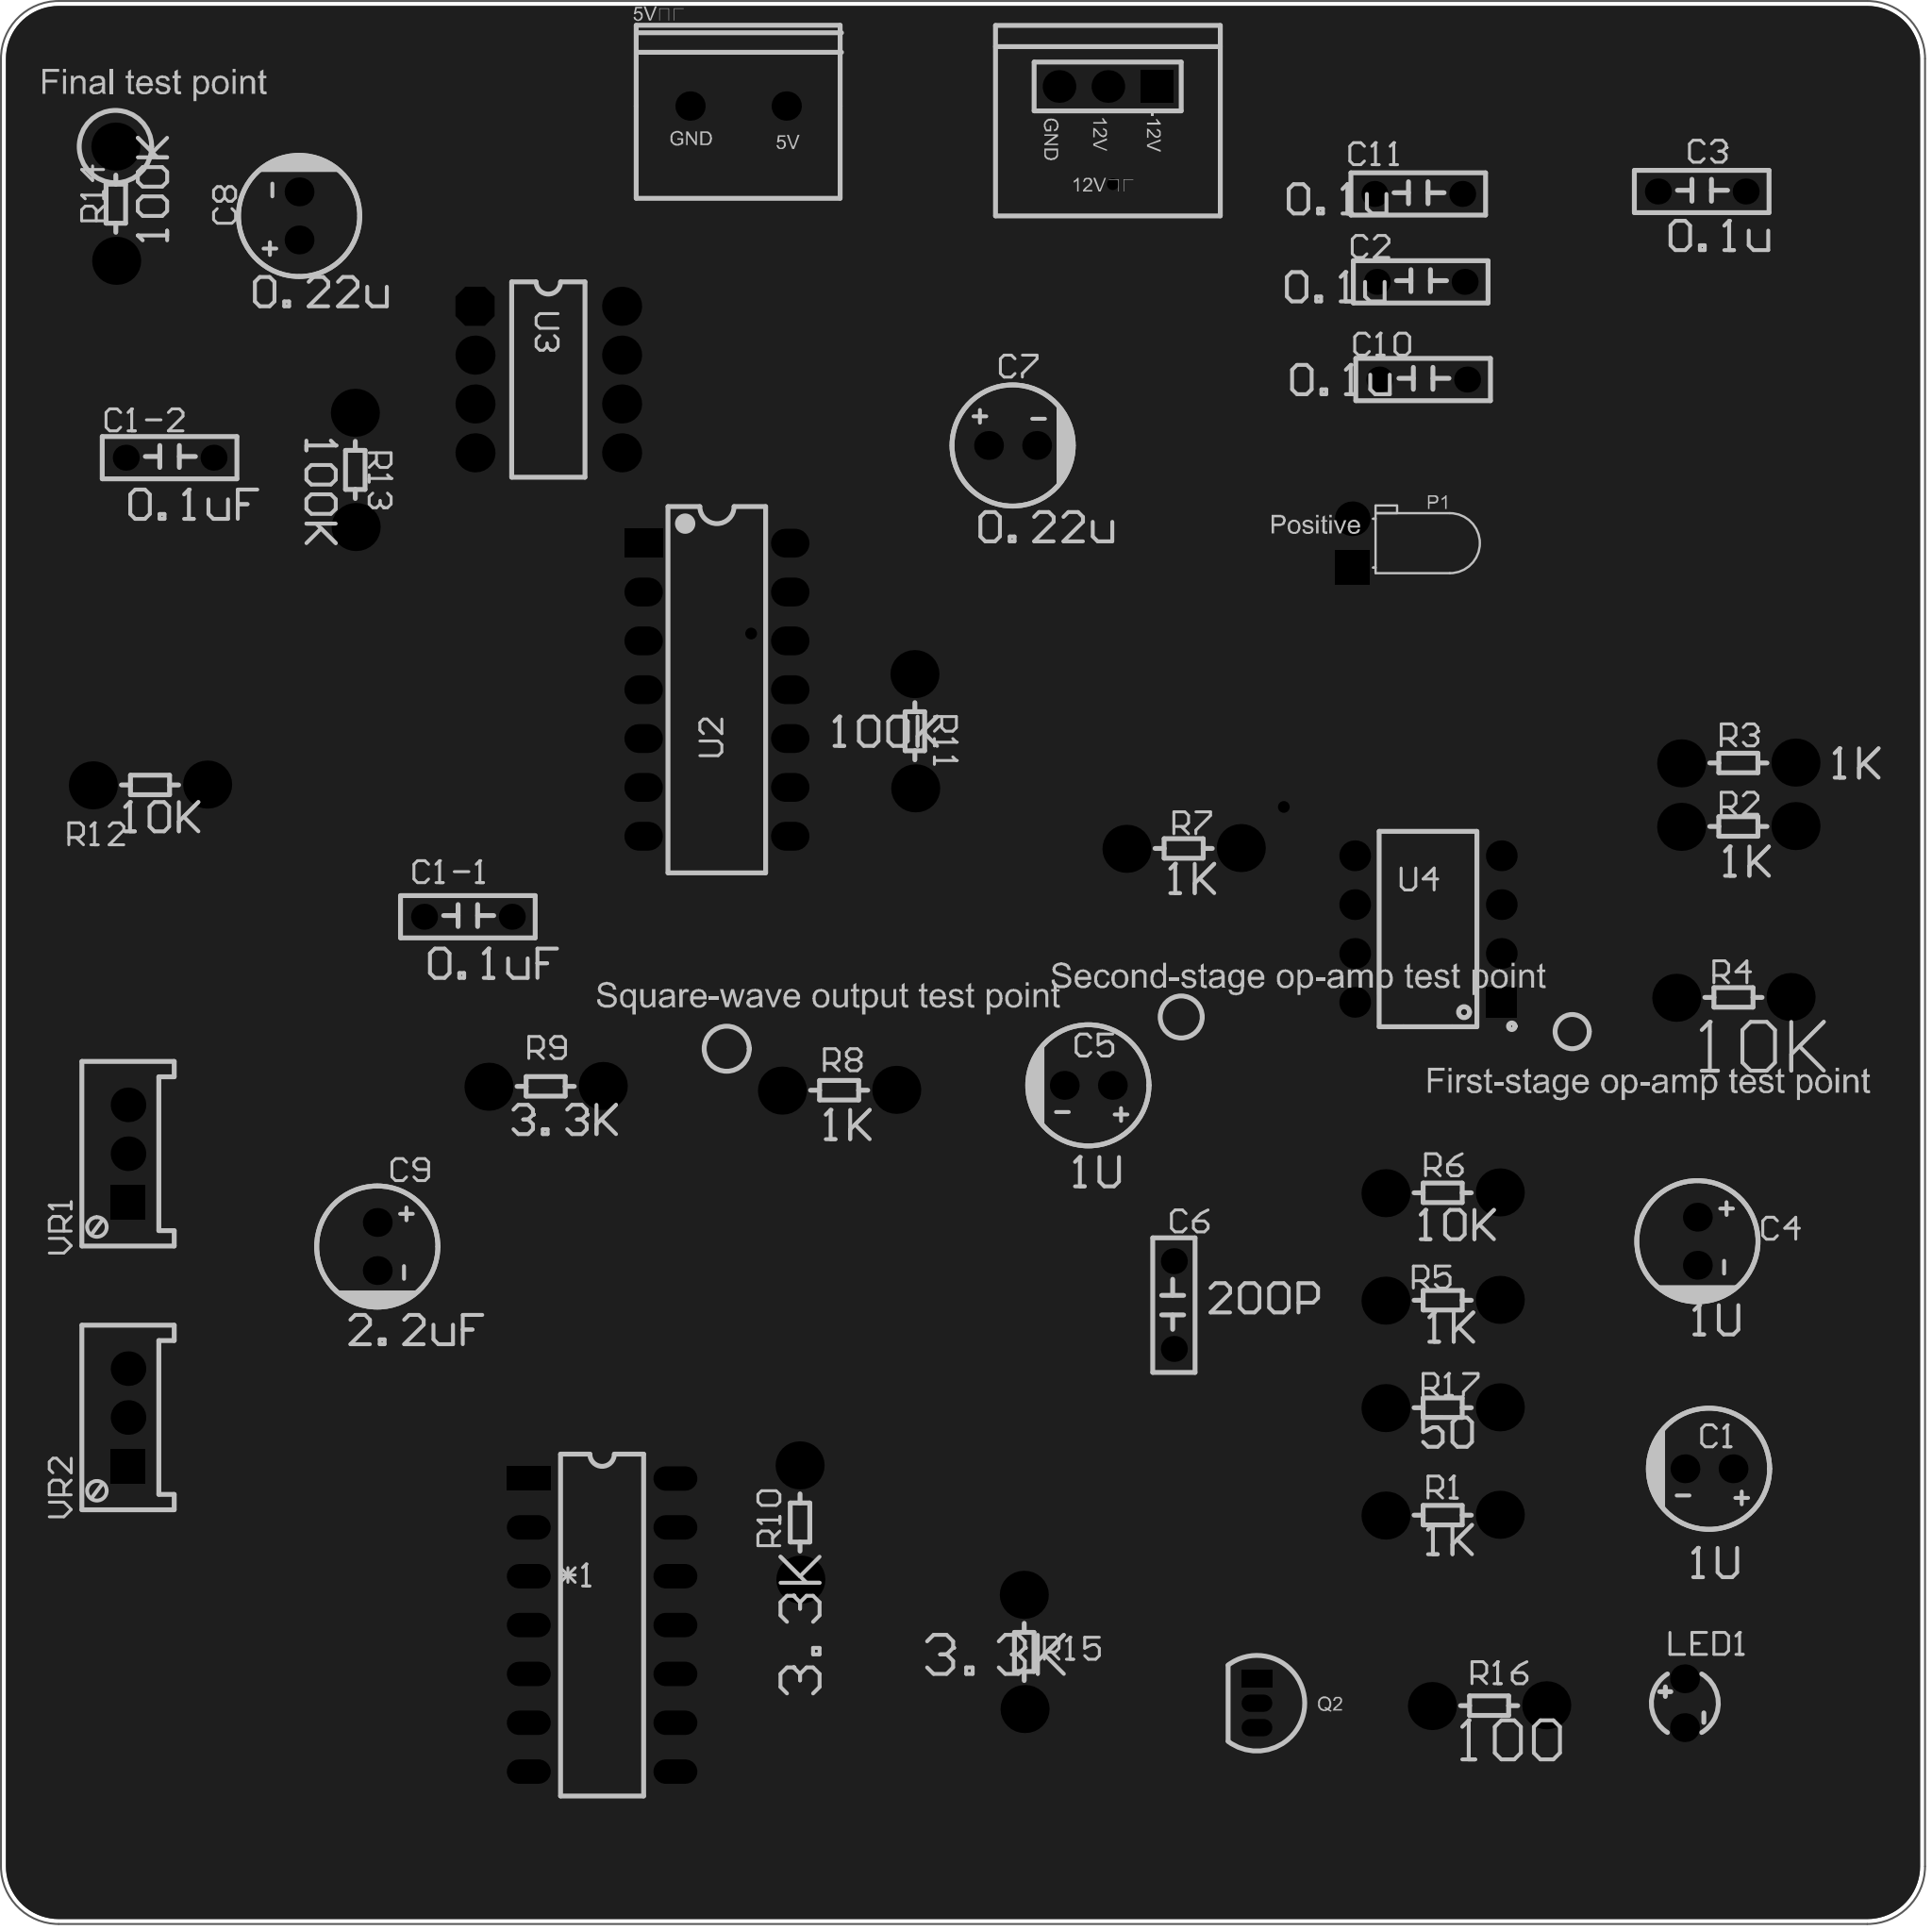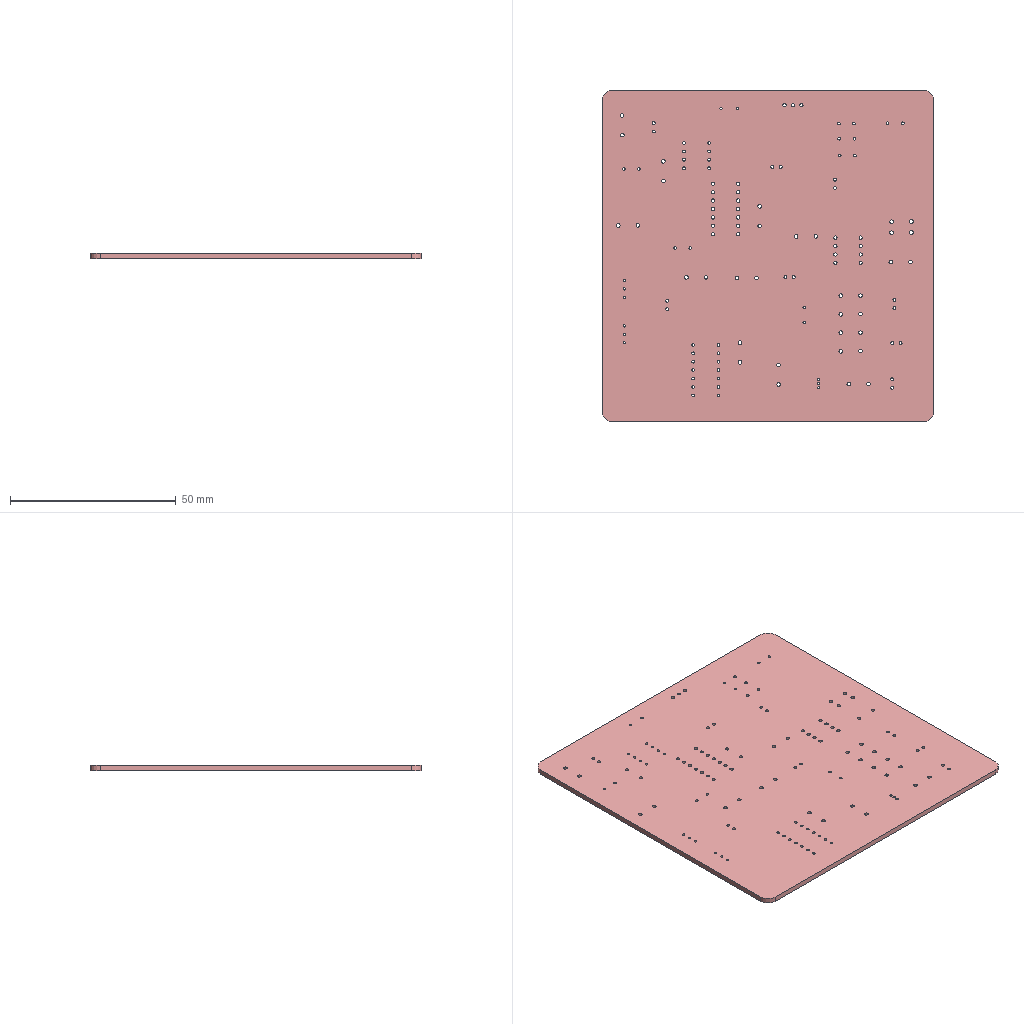Circuit board layout | Altium Designer | box 100 x 100 x 1.6 mm
Layer stack:
# Altium Designer layer stack of  (unit mm; dielectric type: 0 none, 1 core, 2 prepreg, 3 surface material)
index,name,kind,layer,copper_thickness_mm,dielectric_type,dielectric_thickness_mm,dielectric_material,dielectric_constant
0,Top Paste Mask Layer,other,,,,,,
1,Top Silkscreen Layer,other,,,,,,
2,Top Solder Mask Layer,dielectric,,,3,0.01,,3.3
3,Top Layer,copper,Top Layer,0.035,,,,
4,Dielectric1,dielectric,,,3,1.51,FR4,4.5
5,Bottom Layer,copper,Bottom Layer,0.035,,,,
6,Bottom Solder Mask Layer,dielectric,,,3,0.01,,3.3
7,Bottom Silkscreen Layer,other,,,,,,
8,Bottom Paste Mask Layer,other,,,,,,
# drill layer pairs: low layer,high layer
drill_pair,Top Layer,Bottom Layer
Part placement:
Designator,Comment,Layer,Footprint,Center-X(mm),Center-Y(mm),Rotation
C2,,TopLayer,电容直插,155.961,167.132,180
C3,,TopLayer,电容直插,170.566,171.831,180
P1,,TopLayer,LED_D3.0mm_Horizontal_O1.27mm_Z2.0mm,152.4,153.543,90
R1,,TopLayer,D45-V(直插),157.099,102.997,180
R2,,TopLayer,D45-V(直插),172.466,142.113,0
R3,,TopLayer,D45-V(直插),172.466,138.811,180
R4,,TopLayer,D45-V(直插),172.212,129.921,0
R5,,TopLayer,D45-V(直插),157.099,114.173,0
R6,,TopLayer,D45-V(直插),157.099,119.761,0
R7,,TopLayer,D45-V(直插),143.637,137.668,0
C6,,TopLayer,电容直插,143.129,113.924,270
U2,CD4066DN,TopLayer,PDIP-14_L19.3-W6.5-P2.54-LS7.6-BL,119.38,145.923,270
*1,74HC04,TopLayer,DIP14,113.411,97.282,0
C1,220uF,TopLayer,CAP-TH_BD6.3-P2.50-D0.5-FD,170.942,105.41,180
C1-1,,TopLayer,电容直插,106.439,134.116,180
C4,220uF,TopLayer,CAP-TH_BD6.3-P2.50-D0.5-FD,170.337,117.243,270
C5,220uF,TopLayer,CAP-TH_BD6.3-P2.50-D0.5-FD,138.684,125.349,180
C7,220uF,TopLayer,CAP-TH_BD6.3-P2.50-D0.5-FD,134.747,158.623,0
C8,220uF,TopLayer,CAP-TH_BD6.3-P2.50-D0.5-FD,97.663,170.561,90
C1-2,,TopLayer,电容直插,90.937,157.988,180
C10,,TopLayer,电容直插,156.088,162.052,180
C11,,TopLayer,电容直插,155.834,171.704,180
R8,,TopLayer,D45-V(直插),125.73,125.095,0
R9,,TopLayer,D45-V(直插),110.479,125.296,180
R10,,TopLayer,D45-V(直插),123.698,102.616,90
R11,,TopLayer,D45-V(直插),129.667,143.764,90
R12,,TopLayer,D45-V(直插),89.916,140.97,0
R13,,TopLayer,D45-V(直插),100.584,157.353,270
R14,,TopLayer,D45-V(直插),88.138,171.196,90
U3,LF353,TopLayer,DIP-8,110.617,162.052,0
5V输入,5V output,TopLayer,2INT,120.483,176.276,0
12V电源,3PIN,TopLayer,3PIN,139.7,177.292,0
C9,220uF,TopLayer,CAP-TH_BD6.3-P2.50-D0.5-FD,101.727,116.967,270
LED1,3A4GUD,TopLayer,LED-TH_BD3.5-P2.54-RD-GREEN,169.672,93.218,90
Q2,S9018,TopLayer,TO-92-3_L4.9-W3.7-P1.27-L,147.447,93.218,270
R15,,TopLayer,D45-V(直插),135.35,95.885,270
R16,,TopLayer,D45-V(直插),159.512,93.091,0
R17,,TopLayer,D45-V(直插),157.099,108.585,180
U4,,TopLayer,DIP-8_L9.9-W6.4-P2.54-LS7.6-BL,156.337,133.477,90
VR1,101,TopLayer,3296W,88.773,121.793,90
VR2,101,TopLayer,3296W,88.773,108.077,90
Pad and via stacks:
# Altium Designer via and pad stacks of  (unit mm). Each distinct definition once, with the count of objects using it.
# via: kind,start_layer,end_layer,hole_mm,diameter_mm,mode(0 simple;1 top-mid-bottom;2 full stack),diameter_per_layer,count,example_net
# pad: kind,layer,hole_mm,hole_type(0 round;1 square;2 slot),plating,top_size,top_shape(1 round;2 rect;3 octagon;9 rounded rect),mid_size,bottom_size,mode,footprint,size_per_layer,count,example
pad,Multi-Layer,0.81,0,plated,1.35x1.35,1,1.35x1.35,1.35x1.35,0,\u00B5\u00E7\u00C8\u00DD\u00D6\u00B1\u00B2\u00E5,,14,C2.1
pad,Multi-Layer,0.9,0,plated,1.8x1.8,2,1.8x1.8,1.8x1.8,0,LED_D3.0mm_Horizontal_O1.27mm_Z2.0mm,,1,P1.1
pad,Multi-Layer,0.9,0,plated,1.8x1.8,1,1.8x1.8,1.8x1.8,0,LED_D3.0mm_Horizontal_O1.27mm_Z2.0mm,,1,P1.2
pad,Multi-Layer,1.1,2,plated,2.5x2.5,1,2.5x2.5,2.5x2.5,0,D45-V(\u00D6\u00B1\u00B2\u00E5),,34,R1.2
pad,Multi-Layer,1,0,plated,1.5x2,1,1.5x2,1.5x2,0,PDIP-14_L19.3-W6.5-P2.54-LS7.6-BL,,13,U2.8
pad,Multi-Layer,1,0,plated,1.5x2,2,1.5x2,1.5x2,0,PDIP-14_L19.3-W6.5-P2.54-LS7.6-BL,,1,U2.1
pad,Multi-Layer,0.8128,0,plated,2.286x1.27,1,2.286x1.27,2.286x1.27,0,DIP14,,13,*1.8
pad,Multi-Layer,0.8128,0,plated,2.286x1.27,2,2.286x1.27,2.286x1.27,0,DIP14,,1,*1.1
pad,Multi-Layer,0.9,0,plated,1.5x1.5,1,1.5x1.5,1.5x1.5,0,CAP-TH_BD6.3-P2.50-D0.5-FD,,12,C1.2
pad,Multi-Layer,0.8128,0,plated,2.032x2.032,3,2.032x2.032,2.032x2.032,0,DIP-8,,1,U3.1
pad,Multi-Layer,0.8128,0,plated,2.032x2.032,1,1.27x1.27,2.032x2.032,1,DIP-8,,7,U3.2
pad,Multi-Layer,0.762,0,plated,1.524x1.524,1,1.524x1.524,1.524x1.524,0,2INT,,2,5V\u8F93\u5165.1
pad,Multi-Layer,1,0,plated,1.7x1.7,2,1.7x1.7,1.7x1.7,0,3PIN,,1,12V\u7535\u6E90.1
pad,Multi-Layer,1,0,plated,1.7x1.7,1,1.7x1.7,1.7x1.7,0,3PIN,,2,12V\u7535\u6E90.2
pad,Multi-Layer,0.9,0,plated,1.5x1.5,1,1.5x1.5,1.5x1.5,0,LED-TH_BD3.5-P2.54-RD-GREEN,,2,LED1.1
pad,Multi-Layer,0.7,0,plated,0.9x1.6,1,0.9x1.6,0.9x1.6,0,TO-92-3_L4.9-W3.7-P1.27-L,,2,Q2.3
pad,Multi-Layer,0.7,0,plated,0.9x1.6,2,0.9x1.6,0.9x1.6,0,TO-92-3_L4.9-W3.7-P1.27-L,,1,Q2.1
pad,Multi-Layer,1,0,plated,1.6x1.6,1,1.6x1.6,1.6x1.6,0,DIP-8_L9.9-W6.4-P2.54-LS7.6-BL,,7,U4.8
pad,Multi-Layer,1,0,plated,1.6x1.6,2,1.6x1.6,1.6x1.6,0,DIP-8_L9.9-W6.4-P2.54-LS7.6-BL,,1,U4.1
pad,Multi-Layer,0.7,0,plated,1.8x1.8,1,1.8x1.8,1.8x1.8,0,3296W,,4,VR1.3
pad,Multi-Layer,0.7,0,plated,1.8x1.8,2,1.8x1.8,1.8x1.8,0,3296W,,2,VR1.1
via,Top Layer,Bottom Layer,0.3048,0.61,0,,3,12V
Copper pours:
name,layer,net,type(0 solid;1 hatched;2 none)
Top Layer-GND,Top Layer,GND,0
Bottom Layer-GND,Bottom Layer,GND,0
Design rules, without the lines most boards share:
# Altium Designer design rules of  (exported by Altium Designer, unit mm)
# columns: name | kind | enabled | priority | scope1 | scope2 | descriptor | typed fields (field=value)
copperRegion | 20 | enabled | 1 | All | All | Polygon Connect Rule(Direct Connect )(Conductor Width=10mil) (Relief Angle=90 Angle) (Entries=4) (Air Gap Width=10mil) (All),(All) | connect_style(0=relief,1=direct,2=none)=1 relief_conductor_width=0.254 relief_entries=4
solderMaskExpansion | 13 | enabled | 2 | All | All | Solder Mask Expansion (Expansion =2.008mil) (All) | expansion=0.051